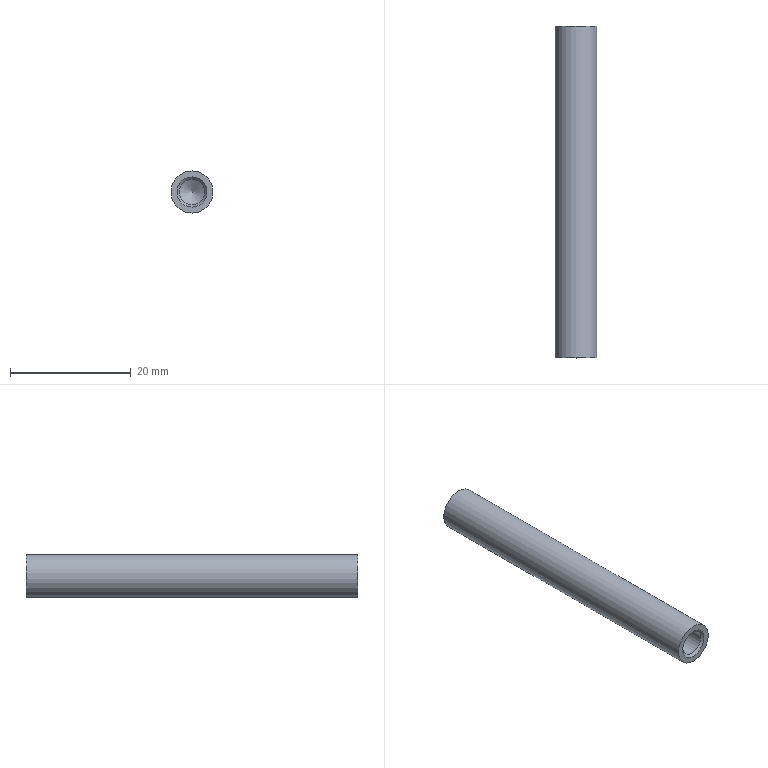Part | STEP file | Coupler copper rod | 1 solid | 9 faces | box 7 x 55 x 7 mm | volume 1826 mm3 | cone 4 | cylinder 3 | plane 2 | commonest cylinder face diameters 4.2 x2 7 x1
STEP:
#1=CARTESIAN_POINT('',(0.,0.,0.));
#2=DIRECTION('',(0.,0.,1.));
#3=DIRECTION('',(1.,0.,0.));
#4=AXIS2_PLACEMENT_3D('',#1,#2,#3);
#5=CARTESIAN_POINT('',(0.,27.5,3.5));
#6=VERTEX_POINT('',#5);
#7=CARTESIAN_POINT('',(0.,27.5,0.));
#8=DIRECTION('',(0.,1.,0.));
#9=DIRECTION('',(0.,0.,1.));
#10=AXIS2_PLACEMENT_3D('',#7,#8,#9);
#11=CIRCLE('',#10,3.5);
#12=CARTESIAN_POINT('',(0.,27.5,0.));
#13=DIRECTION('',(0.,-1.,0.));
#14=DIRECTION('',(0.,0.,-1.));
#15=AXIS2_PLACEMENT_3D('',#12,#13,#14);
#16=CYLINDRICAL_SURFACE('',#15,3.5);
#17=CARTESIAN_POINT('',(9.425,0.));
#18=DIRECTION('',(-1.,0.));
#19=VECTOR('',#18,1.);
#20=LINE('',#17,#19);
#21=(GEOMETRIC_REPRESENTATION_CONTEXT(2)PARAMETRIC_REPRESENTATION_CONTEXT()REPRESENTATION_CONTEXT('',''));
#22=DEFINITIONAL_REPRESENTATION('',(#20),#21);
#23=PCURVE('',#16,#22);
#24=CARTESIAN_POINT('',(0.,27.5,0.));
#25=DIRECTION('',(0.,1.,0.));
#26=DIRECTION('',(0.,0.,1.));
#27=AXIS2_PLACEMENT_3D('',#24,#25,#26);
#28=PLANE('',#27);
#29=CARTESIAN_POINT('',(0.,0.));
#30=DIRECTION('',(1.,0.));
#31=AXIS2_PLACEMENT_2D('',#29,#30);
#32=CIRCLE('',#31,3.5);
#33=(GEOMETRIC_REPRESENTATION_CONTEXT(2)PARAMETRIC_REPRESENTATION_CONTEXT()REPRESENTATION_CONTEXT('',''));
#34=DEFINITIONAL_REPRESENTATION('',(#32),#33);
#35=PCURVE('',#28,#34);
#36=SURFACE_CURVE('',#11,(#23,#35),.PCURVE_S1.);
#37=EDGE_CURVE('',#6,#6,#36,.T.);
#38=ORIENTED_EDGE('',*,*,#37,.F.);
#39=CARTESIAN_POINT('',(0.,-27.5,3.5));
#40=VERTEX_POINT('',#39);
#41=CARTESIAN_POINT('',(0.,27.5,3.5));
#42=CARTESIAN_POINT('',(0.,-27.5,3.5));
#43=B_SPLINE_CURVE_WITH_KNOTS('',1,(#41,#42),.UNSPECIFIED.,.F.,.F.,(2,2),(0.,55.),.PIECEWISE_BEZIER_KNOTS.);
#44=CARTESIAN_POINT('',(9.425,0.));
#45=DIRECTION('',(0.,1.));
#46=VECTOR('',#45,1.);
#47=LINE('',#44,#46);
#48=(GEOMETRIC_REPRESENTATION_CONTEXT(2)PARAMETRIC_REPRESENTATION_CONTEXT()REPRESENTATION_CONTEXT('',''));
#49=DEFINITIONAL_REPRESENTATION('',(#47),#48);
#50=PCURVE('',#16,#49);
#51=CARTESIAN_POINT('',(3.142,0.));
#52=DIRECTION('',(0.,1.));
#53=VECTOR('',#52,1.);
#54=LINE('',#51,#53);
#55=(GEOMETRIC_REPRESENTATION_CONTEXT(2)PARAMETRIC_REPRESENTATION_CONTEXT()REPRESENTATION_CONTEXT('',''));
#56=DEFINITIONAL_REPRESENTATION('',(#54),#55);
#57=PCURVE('',#16,#56);
#58=SEAM_CURVE('',#43,(#50,#57),.PCURVE_S1.);
#59=EDGE_CURVE('',#6,#40,#58,.T.);
#60=ORIENTED_EDGE('',*,*,#59,.T.);
#61=CARTESIAN_POINT('',(0.,-27.5,0.));
#62=DIRECTION('',(0.,1.,0.));
#63=DIRECTION('',(0.,0.,1.));
#64=AXIS2_PLACEMENT_3D('',#61,#62,#63);
#65=CIRCLE('',#64,3.5);
#66=CARTESIAN_POINT('',(9.425,55.));
#67=DIRECTION('',(-1.,0.));
#68=VECTOR('',#67,1.);
#69=LINE('',#66,#68);
#70=(GEOMETRIC_REPRESENTATION_CONTEXT(2)PARAMETRIC_REPRESENTATION_CONTEXT()REPRESENTATION_CONTEXT('',''));
#71=DEFINITIONAL_REPRESENTATION('',(#69),#70);
#72=PCURVE('',#16,#71);
#73=CARTESIAN_POINT('',(0.,-27.5,0.));
#74=DIRECTION('',(0.,1.,0.));
#75=DIRECTION('',(0.,0.,1.));
#76=AXIS2_PLACEMENT_3D('',#73,#74,#75);
#77=PLANE('',#76);
#78=CARTESIAN_POINT('',(0.,0.));
#79=DIRECTION('',(1.,0.));
#80=AXIS2_PLACEMENT_2D('',#78,#79);
#81=CIRCLE('',#80,3.5);
#82=(GEOMETRIC_REPRESENTATION_CONTEXT(2)PARAMETRIC_REPRESENTATION_CONTEXT()REPRESENTATION_CONTEXT('',''));
#83=DEFINITIONAL_REPRESENTATION('',(#81),#82);
#84=PCURVE('',#77,#83);
#85=SURFACE_CURVE('',#65,(#72,#84),.PCURVE_S1.);
#86=EDGE_CURVE('',#40,#40,#85,.T.);
#87=ORIENTED_EDGE('',*,*,#86,.T.);
#88=ORIENTED_EDGE('',*,*,#59,.F.);
#89=EDGE_LOOP('',(#38,#60,#87,#88));
#90=FACE_BOUND('',#89,.T.);
#91=ADVANCED_FACE('',(#90),#16,.T.);
#92=CARTESIAN_POINT('',(0.,27.5,2.5));
#93=VERTEX_POINT('',#92);
#94=CARTESIAN_POINT('',(0.,27.5,0.));
#95=DIRECTION('',(0.,1.,0.));
#96=DIRECTION('',(0.,0.,1.));
#97=AXIS2_PLACEMENT_3D('',#94,#95,#96);
#98=CIRCLE('',#97,2.5);
#99=CARTESIAN_POINT('',(0.,0.));
#100=DIRECTION('',(1.,0.));
#101=AXIS2_PLACEMENT_2D('',#99,#100);
#102=CIRCLE('',#101,2.5);
#103=(GEOMETRIC_REPRESENTATION_CONTEXT(2)PARAMETRIC_REPRESENTATION_CONTEXT()REPRESENTATION_CONTEXT('',''));
#104=DEFINITIONAL_REPRESENTATION('',(#102),#103);
#105=PCURVE('',#28,#104);
#106=CARTESIAN_POINT('',(0.,25.,0.));
#107=DIRECTION('',(0.,1.,0.));
#108=DIRECTION('',(1.,0.,0.));
#109=AXIS2_PLACEMENT_3D('',#106,#107,#108);
#110=CONICAL_SURFACE('',#109,0.,0.7854);
#111=CARTESIAN_POINT('',(4.712,2.5));
#112=DIRECTION('',(1.,0.));
#113=VECTOR('',#112,1.);
#114=LINE('',#111,#113);
#115=(GEOMETRIC_REPRESENTATION_CONTEXT(2)PARAMETRIC_REPRESENTATION_CONTEXT()REPRESENTATION_CONTEXT('',''));
#116=DEFINITIONAL_REPRESENTATION('',(#114),#115);
#117=PCURVE('',#110,#116);
#118=SURFACE_CURVE('',#98,(#105,#117),.PCURVE_S1.);
#119=EDGE_CURVE('',#93,#93,#118,.T.);
#120=ORIENTED_EDGE('',*,*,#119,.F.);
#121=EDGE_LOOP('',(#120));
#122=FACE_BOUND('',#121,.T.);
#123=ORIENTED_EDGE('',*,*,#37,.T.);
#124=EDGE_LOOP('',(#123));
#125=FACE_BOUND('',#124,.T.);
#126=ADVANCED_FACE('',(#122,#125),#28,.T.);
#127=CARTESIAN_POINT('',(0.,-27.5,2.5));
#128=VERTEX_POINT('',#127);
#129=CARTESIAN_POINT('',(0.,-27.5,0.));
#130=DIRECTION('',(0.,1.,0.));
#131=DIRECTION('',(0.,0.,1.));
#132=AXIS2_PLACEMENT_3D('',#129,#130,#131);
#133=CIRCLE('',#132,2.5);
#134=CARTESIAN_POINT('',(0.,0.));
#135=DIRECTION('',(1.,0.));
#136=AXIS2_PLACEMENT_2D('',#134,#135);
#137=CIRCLE('',#136,2.5);
#138=(GEOMETRIC_REPRESENTATION_CONTEXT(2)PARAMETRIC_REPRESENTATION_CONTEXT()REPRESENTATION_CONTEXT('',''));
#139=DEFINITIONAL_REPRESENTATION('',(#137),#138);
#140=PCURVE('',#77,#139);
#141=CARTESIAN_POINT('',(0.,-25.,0.));
#142=DIRECTION('',(0.,-1.,0.));
#143=DIRECTION('',(-1.,0.,0.));
#144=AXIS2_PLACEMENT_3D('',#141,#142,#143);
#145=CONICAL_SURFACE('',#144,0.,0.7854);
#146=CARTESIAN_POINT('',(10.996,2.5));
#147=DIRECTION('',(-1.,0.));
#148=VECTOR('',#147,1.);
#149=LINE('',#146,#148);
#150=(GEOMETRIC_REPRESENTATION_CONTEXT(2)PARAMETRIC_REPRESENTATION_CONTEXT()REPRESENTATION_CONTEXT('',''));
#151=DEFINITIONAL_REPRESENTATION('',(#149),#150);
#152=PCURVE('',#145,#151);
#153=SURFACE_CURVE('',#133,(#140,#152),.PCURVE_S1.);
#154=EDGE_CURVE('',#128,#128,#153,.T.);
#155=ORIENTED_EDGE('',*,*,#154,.T.);
#156=EDGE_LOOP('',(#155));
#157=FACE_BOUND('',#156,.T.);
#158=ORIENTED_EDGE('',*,*,#86,.F.);
#159=EDGE_LOOP('',(#158));
#160=FACE_BOUND('',#159,.T.);
#161=ADVANCED_FACE('',(#157,#160),#77,.F.);
#162=ORIENTED_EDGE('',*,*,#154,.T.);
#163=CARTESIAN_POINT('',(0.,-27.1,2.1));
#164=VERTEX_POINT('',#163);
#165=CARTESIAN_POINT('',(0.,-27.1,2.1));
#166=CARTESIAN_POINT('',(0.,-27.5,2.5));
#167=B_SPLINE_CURVE_WITH_KNOTS('',1,(#165,#166),.UNSPECIFIED.,.F.,.F.,(2,2),(2.97,3.536),.PIECEWISE_BEZIER_KNOTS.);
#168=CARTESIAN_POINT('',(4.712,0.));
#169=DIRECTION('',(0.,1.));
#170=VECTOR('',#169,1.);
#171=LINE('',#168,#170);
#172=(GEOMETRIC_REPRESENTATION_CONTEXT(2)PARAMETRIC_REPRESENTATION_CONTEXT()REPRESENTATION_CONTEXT('',''));
#173=DEFINITIONAL_REPRESENTATION('',(#171),#172);
#174=PCURVE('',#145,#173);
#175=CARTESIAN_POINT('',(10.996,0.));
#176=DIRECTION('',(0.,1.));
#177=VECTOR('',#176,1.);
#178=LINE('',#175,#177);
#179=(GEOMETRIC_REPRESENTATION_CONTEXT(2)PARAMETRIC_REPRESENTATION_CONTEXT()REPRESENTATION_CONTEXT('',''));
#180=DEFINITIONAL_REPRESENTATION('',(#178),#179);
#181=PCURVE('',#145,#180);
#182=SEAM_CURVE('',#167,(#174,#181),.PCURVE_S1.);
#183=EDGE_CURVE('',#164,#128,#182,.T.);
#184=ORIENTED_EDGE('',*,*,#183,.F.);
#185=CARTESIAN_POINT('',(0.,-27.1,-2.1));
#186=VERTEX_POINT('',#185);
#187=CARTESIAN_POINT('',(0.,-27.1,0.));
#188=DIRECTION('',(0.,-1.,0.));
#189=DIRECTION('',(0.,0.,-1.));
#190=AXIS2_PLACEMENT_3D('',#187,#188,#189);
#191=CIRCLE('',#190,2.1);
#192=CARTESIAN_POINT('',(1.571,2.1));
#193=DIRECTION('',(1.,0.));
#194=VECTOR('',#193,1.);
#195=LINE('',#192,#194);
#196=(GEOMETRIC_REPRESENTATION_CONTEXT(2)PARAMETRIC_REPRESENTATION_CONTEXT()REPRESENTATION_CONTEXT('',''));
#197=DEFINITIONAL_REPRESENTATION('',(#195),#196);
#198=PCURVE('',#145,#197);
#199=CARTESIAN_POINT('',(0.,-27.5,0.));
#200=DIRECTION('',(0.,1.,0.));
#201=DIRECTION('',(0.,0.,1.));
#202=AXIS2_PLACEMENT_3D('',#199,#200,#201);
#203=CYLINDRICAL_SURFACE('',#202,2.1);
#204=CARTESIAN_POINT('',(9.425,0.4));
#205=DIRECTION('',(-1.,0.));
#206=VECTOR('',#205,1.);
#207=LINE('',#204,#206);
#208=(GEOMETRIC_REPRESENTATION_CONTEXT(2)PARAMETRIC_REPRESENTATION_CONTEXT()REPRESENTATION_CONTEXT('',''));
#209=DEFINITIONAL_REPRESENTATION('',(#207),#208);
#210=PCURVE('',#203,#209);
#211=SURFACE_CURVE('',#191,(#198,#210),.PCURVE_S1.);
#212=EDGE_CURVE('',#164,#186,#211,.T.);
#213=ORIENTED_EDGE('',*,*,#212,.T.);
#214=CARTESIAN_POINT('',(0.,-27.1,0.));
#215=DIRECTION('',(0.,-1.,0.));
#216=DIRECTION('',(0.,0.,-1.));
#217=AXIS2_PLACEMENT_3D('',#214,#215,#216);
#218=CIRCLE('',#217,2.1);
#219=CARTESIAN_POINT('',(7.854,2.1));
#220=DIRECTION('',(1.,0.));
#221=VECTOR('',#220,1.);
#222=LINE('',#219,#221);
#223=(GEOMETRIC_REPRESENTATION_CONTEXT(2)PARAMETRIC_REPRESENTATION_CONTEXT()REPRESENTATION_CONTEXT('',''));
#224=DEFINITIONAL_REPRESENTATION('',(#222),#223);
#225=PCURVE('',#145,#224);
#226=CARTESIAN_POINT('',(3.142,0.4));
#227=DIRECTION('',(-1.,0.));
#228=VECTOR('',#227,1.);
#229=LINE('',#226,#228);
#230=(GEOMETRIC_REPRESENTATION_CONTEXT(2)PARAMETRIC_REPRESENTATION_CONTEXT()REPRESENTATION_CONTEXT('',''));
#231=DEFINITIONAL_REPRESENTATION('',(#229),#230);
#232=PCURVE('',#203,#231);
#233=SURFACE_CURVE('',#218,(#225,#232),.PCURVE_S1.);
#234=EDGE_CURVE('',#186,#164,#233,.T.);
#235=ORIENTED_EDGE('',*,*,#234,.T.);
#236=ORIENTED_EDGE('',*,*,#183,.T.);
#237=EDGE_LOOP('',(#162,#184,#213,#235,#236));
#238=FACE_BOUND('',#237,.F.);
#239=ADVANCED_FACE('',(#238),#145,.F.);
#240=CARTESIAN_POINT('',(0.,-17.5,-2.1));
#241=VERTEX_POINT('',#240);
#242=CARTESIAN_POINT('',(0.,-17.5,2.1));
#243=VERTEX_POINT('',#242);
#244=CARTESIAN_POINT('',(0.,-17.5,0.));
#245=DIRECTION('',(0.,-1.,0.));
#246=DIRECTION('',(0.,0.,1.));
#247=AXIS2_PLACEMENT_3D('',#244,#245,#246);
#248=CIRCLE('',#247,2.1);
#249=CARTESIAN_POINT('',(0.,-17.5,0.));
#250=DIRECTION('',(0.,-1.,0.));
#251=DIRECTION('',(0.,0.,-1.));
#252=AXIS2_PLACEMENT_3D('',#249,#250,#251);
#253=CONICAL_SURFACE('',#252,2.1,1.03);
#254=CARTESIAN_POINT('',(-3.142,0.));
#255=DIRECTION('',(1.,0.));
#256=VECTOR('',#255,1.);
#257=LINE('',#254,#256);
#258=(GEOMETRIC_REPRESENTATION_CONTEXT(2)PARAMETRIC_REPRESENTATION_CONTEXT()REPRESENTATION_CONTEXT('',''));
#259=DEFINITIONAL_REPRESENTATION('',(#257),#258);
#260=PCURVE('',#253,#259);
#261=CARTESIAN_POINT('',(6.283,10.));
#262=DIRECTION('',(-1.,0.));
#263=VECTOR('',#262,1.);
#264=LINE('',#261,#263);
#265=(GEOMETRIC_REPRESENTATION_CONTEXT(2)PARAMETRIC_REPRESENTATION_CONTEXT()REPRESENTATION_CONTEXT('',''));
#266=DEFINITIONAL_REPRESENTATION('',(#264),#265);
#267=PCURVE('',#203,#266);
#268=SURFACE_CURVE('',#248,(#260,#267),.PCURVE_S1.);
#269=EDGE_CURVE('',#241,#243,#268,.T.);
#270=ORIENTED_EDGE('',*,*,#269,.F.);
#271=CARTESIAN_POINT('',(0.,-16.238,0.));
#272=VERTEX_POINT('',#271);
#273=CARTESIAN_POINT('',(0.,-16.238,0.));
#274=CARTESIAN_POINT('',(0.,-17.5,-2.1));
#275=B_SPLINE_CURVE_WITH_KNOTS('',1,(#273,#274),.UNSPECIFIED.,.F.,.F.,(2,2),(-2.45,0.),.PIECEWISE_BEZIER_KNOTS.);
#276=CARTESIAN_POINT('',(0.,0.));
#277=DIRECTION('',(0.,1.));
#278=VECTOR('',#277,1.);
#279=LINE('',#276,#278);
#280=(GEOMETRIC_REPRESENTATION_CONTEXT(2)PARAMETRIC_REPRESENTATION_CONTEXT()REPRESENTATION_CONTEXT('',''));
#281=DEFINITIONAL_REPRESENTATION('',(#279),#280);
#282=PCURVE('',#253,#281);
#283=CARTESIAN_POINT('',(6.283,0.));
#284=DIRECTION('',(0.,1.));
#285=VECTOR('',#284,1.);
#286=LINE('',#283,#285);
#287=(GEOMETRIC_REPRESENTATION_CONTEXT(2)PARAMETRIC_REPRESENTATION_CONTEXT()REPRESENTATION_CONTEXT('',''));
#288=DEFINITIONAL_REPRESENTATION('',(#286),#287);
#289=PCURVE('',#253,#288);
#290=SEAM_CURVE('',#275,(#282,#289),.PCURVE_S1.);
#291=EDGE_CURVE('',#272,#241,#290,.T.);
#292=ORIENTED_EDGE('',*,*,#291,.F.);
#293=ORIENTED_EDGE('',*,*,#291,.T.);
#294=CARTESIAN_POINT('',(0.,-17.5,0.));
#295=DIRECTION('',(0.,-1.,0.));
#296=DIRECTION('',(0.,0.,1.));
#297=AXIS2_PLACEMENT_3D('',#294,#295,#296);
#298=CIRCLE('',#297,2.1);
#299=CARTESIAN_POINT('',(3.142,0.));
#300=DIRECTION('',(1.,0.));
#301=VECTOR('',#300,1.);
#302=LINE('',#299,#301);
#303=(GEOMETRIC_REPRESENTATION_CONTEXT(2)PARAMETRIC_REPRESENTATION_CONTEXT()REPRESENTATION_CONTEXT('',''));
#304=DEFINITIONAL_REPRESENTATION('',(#302),#303);
#305=PCURVE('',#253,#304);
#306=CARTESIAN_POINT('',(6.283,10.));
#307=DIRECTION('',(-1.,0.));
#308=VECTOR('',#307,1.);
#309=LINE('',#306,#308);
#310=(GEOMETRIC_REPRESENTATION_CONTEXT(2)PARAMETRIC_REPRESENTATION_CONTEXT()REPRESENTATION_CONTEXT('',''));
#311=DEFINITIONAL_REPRESENTATION('',(#309),#310);
#312=PCURVE('',#203,#311);
#313=SURFACE_CURVE('',#298,(#305,#312),.PCURVE_S1.);
#314=EDGE_CURVE('',#243,#241,#313,.T.);
#315=ORIENTED_EDGE('',*,*,#314,.F.);
#316=EDGE_LOOP('',(#270,#292,#293,#315));
#317=FACE_BOUND('',#316,.F.);
#318=ADVANCED_FACE('',(#317),#253,.F.);
#319=ORIENTED_EDGE('',*,*,#212,.F.);
#320=CARTESIAN_POINT('',(0.,-27.1,2.1));
#321=CARTESIAN_POINT('',(0.,-17.5,2.1));
#322=B_SPLINE_CURVE_WITH_KNOTS('',1,(#320,#321),.UNSPECIFIED.,.F.,.F.,(2,2),(0.4,10.),.PIECEWISE_BEZIER_KNOTS.);
#323=CARTESIAN_POINT('',(6.283,0.));
#324=DIRECTION('',(0.,1.));
#325=VECTOR('',#324,1.);
#326=LINE('',#323,#325);
#327=(GEOMETRIC_REPRESENTATION_CONTEXT(2)PARAMETRIC_REPRESENTATION_CONTEXT()REPRESENTATION_CONTEXT('',''));
#328=DEFINITIONAL_REPRESENTATION('',(#326),#327);
#329=PCURVE('',#203,#328);
#330=CARTESIAN_POINT('',(0.,0.));
#331=DIRECTION('',(0.,1.));
#332=VECTOR('',#331,1.);
#333=LINE('',#330,#332);
#334=(GEOMETRIC_REPRESENTATION_CONTEXT(2)PARAMETRIC_REPRESENTATION_CONTEXT()REPRESENTATION_CONTEXT('',''));
#335=DEFINITIONAL_REPRESENTATION('',(#333),#334);
#336=PCURVE('',#203,#335);
#337=SEAM_CURVE('',#322,(#329,#336),.PCURVE_S1.);
#338=EDGE_CURVE('',#164,#243,#337,.T.);
#339=ORIENTED_EDGE('',*,*,#338,.T.);
#340=ORIENTED_EDGE('',*,*,#314,.T.);
#341=ORIENTED_EDGE('',*,*,#269,.T.);
#342=ORIENTED_EDGE('',*,*,#338,.F.);
#343=ORIENTED_EDGE('',*,*,#234,.F.);
#344=EDGE_LOOP('',(#319,#339,#340,#341,#342,#343));
#345=FACE_BOUND('',#344,.F.);
#346=ADVANCED_FACE('',(#345),#203,.F.);
#347=ORIENTED_EDGE('',*,*,#119,.F.);
#348=CARTESIAN_POINT('',(0.,27.1,2.1));
#349=VERTEX_POINT('',#348);
#350=CARTESIAN_POINT('',(0.,27.1,2.1));
#351=CARTESIAN_POINT('',(0.,27.5,2.5));
#352=B_SPLINE_CURVE_WITH_KNOTS('',1,(#350,#351),.UNSPECIFIED.,.F.,.F.,(2,2),(2.97,3.536),.PIECEWISE_BEZIER_KNOTS.);
#353=CARTESIAN_POINT('',(4.712,0.));
#354=DIRECTION('',(0.,1.));
#355=VECTOR('',#354,1.);
#356=LINE('',#353,#355);
#357=(GEOMETRIC_REPRESENTATION_CONTEXT(2)PARAMETRIC_REPRESENTATION_CONTEXT()REPRESENTATION_CONTEXT('',''));
#358=DEFINITIONAL_REPRESENTATION('',(#356),#357);
#359=PCURVE('',#110,#358);
#360=CARTESIAN_POINT('',(10.996,0.));
#361=DIRECTION('',(0.,1.));
#362=VECTOR('',#361,1.);
#363=LINE('',#360,#362);
#364=(GEOMETRIC_REPRESENTATION_CONTEXT(2)PARAMETRIC_REPRESENTATION_CONTEXT()REPRESENTATION_CONTEXT('',''));
#365=DEFINITIONAL_REPRESENTATION('',(#363),#364);
#366=PCURVE('',#110,#365);
#367=SEAM_CURVE('',#352,(#359,#366),.PCURVE_S1.);
#368=EDGE_CURVE('',#349,#93,#367,.T.);
#369=ORIENTED_EDGE('',*,*,#368,.F.);
#370=CARTESIAN_POINT('',(0.,27.1,0.));
#371=DIRECTION('',(0.,1.,0.));
#372=DIRECTION('',(0.,0.,1.));
#373=AXIS2_PLACEMENT_3D('',#370,#371,#372);
#374=CIRCLE('',#373,2.1);
#375=CARTESIAN_POINT('',(4.712,2.1));
#376=DIRECTION('',(1.,0.));
#377=VECTOR('',#376,1.);
#378=LINE('',#375,#377);
#379=(GEOMETRIC_REPRESENTATION_CONTEXT(2)PARAMETRIC_REPRESENTATION_CONTEXT()REPRESENTATION_CONTEXT('',''));
#380=DEFINITIONAL_REPRESENTATION('',(#378),#379);
#381=PCURVE('',#110,#380);
#382=CARTESIAN_POINT('',(0.,27.5,0.));
#383=DIRECTION('',(0.,-1.,0.));
#384=DIRECTION('',(0.,0.,-1.));
#385=AXIS2_PLACEMENT_3D('',#382,#383,#384);
#386=CYLINDRICAL_SURFACE('',#385,2.1);
#387=CARTESIAN_POINT('',(9.425,0.4));
#388=DIRECTION('',(-1.,0.));
#389=VECTOR('',#388,1.);
#390=LINE('',#387,#389);
#391=(GEOMETRIC_REPRESENTATION_CONTEXT(2)PARAMETRIC_REPRESENTATION_CONTEXT()REPRESENTATION_CONTEXT('',''));
#392=DEFINITIONAL_REPRESENTATION('',(#390),#391);
#393=PCURVE('',#386,#392);
#394=SURFACE_CURVE('',#374,(#381,#393),.PCURVE_S1.);
#395=EDGE_CURVE('',#349,#349,#394,.T.);
#396=ORIENTED_EDGE('',*,*,#395,.T.);
#397=ORIENTED_EDGE('',*,*,#368,.T.);
#398=EDGE_LOOP('',(#347,#369,#396,#397));
#399=FACE_BOUND('',#398,.F.);
#400=ADVANCED_FACE('',(#399),#110,.F.);
#401=CARTESIAN_POINT('',(0.,17.5,2.1));
#402=VERTEX_POINT('',#401);
#403=CARTESIAN_POINT('',(0.,17.5,-2.1));
#404=VERTEX_POINT('',#403);
#405=CARTESIAN_POINT('',(0.,17.5,0.));
#406=DIRECTION('',(0.,1.,0.));
#407=DIRECTION('',(0.,0.,-1.));
#408=AXIS2_PLACEMENT_3D('',#405,#406,#407);
#409=CIRCLE('',#408,2.1);
#410=CARTESIAN_POINT('',(0.,17.5,0.));
#411=DIRECTION('',(0.,1.,0.));
#412=DIRECTION('',(0.,0.,1.));
#413=AXIS2_PLACEMENT_3D('',#410,#411,#412);
#414=CONICAL_SURFACE('',#413,2.1,1.03);
#415=CARTESIAN_POINT('',(-3.142,0.));
#416=DIRECTION('',(1.,0.));
#417=VECTOR('',#416,1.);
#418=LINE('',#415,#417);
#419=(GEOMETRIC_REPRESENTATION_CONTEXT(2)PARAMETRIC_REPRESENTATION_CONTEXT()REPRESENTATION_CONTEXT('',''));
#420=DEFINITIONAL_REPRESENTATION('',(#418),#419);
#421=PCURVE('',#414,#420);
#422=CARTESIAN_POINT('',(12.566,10.));
#423=DIRECTION('',(-1.,0.));
#424=VECTOR('',#423,1.);
#425=LINE('',#422,#424);
#426=(GEOMETRIC_REPRESENTATION_CONTEXT(2)PARAMETRIC_REPRESENTATION_CONTEXT()REPRESENTATION_CONTEXT('',''));
#427=DEFINITIONAL_REPRESENTATION('',(#425),#426);
#428=PCURVE('',#386,#427);
#429=SURFACE_CURVE('',#409,(#421,#428),.PCURVE_S1.);
#430=EDGE_CURVE('',#402,#404,#429,.T.);
#431=ORIENTED_EDGE('',*,*,#430,.F.);
#432=CARTESIAN_POINT('',(0.,16.238,0.));
#433=VERTEX_POINT('',#432);
#434=CARTESIAN_POINT('',(0.,16.238,0.));
#435=CARTESIAN_POINT('',(0.,17.5,2.1));
#436=B_SPLINE_CURVE_WITH_KNOTS('',1,(#434,#435),.UNSPECIFIED.,.F.,.F.,(2,2),(-2.45,0.),.PIECEWISE_BEZIER_KNOTS.);
#437=CARTESIAN_POINT('',(0.,0.));
#438=DIRECTION('',(0.,1.));
#439=VECTOR('',#438,1.);
#440=LINE('',#437,#439);
#441=(GEOMETRIC_REPRESENTATION_CONTEXT(2)PARAMETRIC_REPRESENTATION_CONTEXT()REPRESENTATION_CONTEXT('',''));
#442=DEFINITIONAL_REPRESENTATION('',(#440),#441);
#443=PCURVE('',#414,#442);
#444=CARTESIAN_POINT('',(6.283,0.));
#445=DIRECTION('',(0.,1.));
#446=VECTOR('',#445,1.);
#447=LINE('',#444,#446);
#448=(GEOMETRIC_REPRESENTATION_CONTEXT(2)PARAMETRIC_REPRESENTATION_CONTEXT()REPRESENTATION_CONTEXT('',''));
#449=DEFINITIONAL_REPRESENTATION('',(#447),#448);
#450=PCURVE('',#414,#449);
#451=SEAM_CURVE('',#436,(#443,#450),.PCURVE_S1.);
#452=EDGE_CURVE('',#433,#402,#451,.T.);
#453=ORIENTED_EDGE('',*,*,#452,.F.);
#454=ORIENTED_EDGE('',*,*,#452,.T.);
#455=CARTESIAN_POINT('',(0.,17.5,0.));
#456=DIRECTION('',(0.,1.,0.));
#457=DIRECTION('',(0.,0.,-1.));
#458=AXIS2_PLACEMENT_3D('',#455,#456,#457);
#459=CIRCLE('',#458,2.1);
#460=CARTESIAN_POINT('',(3.142,0.));
#461=DIRECTION('',(1.,0.));
#462=VECTOR('',#461,1.);
#463=LINE('',#460,#462);
#464=(GEOMETRIC_REPRESENTATION_CONTEXT(2)PARAMETRIC_REPRESENTATION_CONTEXT()REPRESENTATION_CONTEXT('',''));
#465=DEFINITIONAL_REPRESENTATION('',(#463),#464);
#466=PCURVE('',#414,#465);
#467=CARTESIAN_POINT('',(6.283,10.));
#468=DIRECTION('',(-1.,0.));
#469=VECTOR('',#468,1.);
#470=LINE('',#467,#469);
#471=(GEOMETRIC_REPRESENTATION_CONTEXT(2)PARAMETRIC_REPRESENTATION_CONTEXT()REPRESENTATION_CONTEXT('',''));
#472=DEFINITIONAL_REPRESENTATION('',(#470),#471);
#473=PCURVE('',#386,#472);
#474=SURFACE_CURVE('',#459,(#466,#473),.PCURVE_S1.);
#475=EDGE_CURVE('',#404,#402,#474,.T.);
#476=ORIENTED_EDGE('',*,*,#475,.F.);
#477=EDGE_LOOP('',(#431,#453,#454,#476));
#478=FACE_BOUND('',#477,.F.);
#479=ADVANCED_FACE('',(#478),#414,.F.);
#480=ORIENTED_EDGE('',*,*,#395,.F.);
#481=CARTESIAN_POINT('',(0.,27.1,2.1));
#482=CARTESIAN_POINT('',(0.,17.5,2.1));
#483=B_SPLINE_CURVE_WITH_KNOTS('',1,(#481,#482),.UNSPECIFIED.,.F.,.F.,(2,2),(0.4,10.),.PIECEWISE_BEZIER_KNOTS.);
#484=CARTESIAN_POINT('',(9.425,0.));
#485=DIRECTION('',(0.,1.));
#486=VECTOR('',#485,1.);
#487=LINE('',#484,#486);
#488=(GEOMETRIC_REPRESENTATION_CONTEXT(2)PARAMETRIC_REPRESENTATION_CONTEXT()REPRESENTATION_CONTEXT('',''));
#489=DEFINITIONAL_REPRESENTATION('',(#487),#488);
#490=PCURVE('',#386,#489);
#491=CARTESIAN_POINT('',(3.142,0.));
#492=DIRECTION('',(0.,1.));
#493=VECTOR('',#492,1.);
#494=LINE('',#491,#493);
#495=(GEOMETRIC_REPRESENTATION_CONTEXT(2)PARAMETRIC_REPRESENTATION_CONTEXT()REPRESENTATION_CONTEXT('',''));
#496=DEFINITIONAL_REPRESENTATION('',(#494),#495);
#497=PCURVE('',#386,#496);
#498=SEAM_CURVE('',#483,(#490,#497),.PCURVE_S1.);
#499=EDGE_CURVE('',#349,#402,#498,.T.);
#500=ORIENTED_EDGE('',*,*,#499,.T.);
#501=ORIENTED_EDGE('',*,*,#430,.T.);
#502=ORIENTED_EDGE('',*,*,#475,.T.);
#503=ORIENTED_EDGE('',*,*,#499,.F.);
#504=EDGE_LOOP('',(#480,#500,#501,#502,#503));
#505=FACE_BOUND('',#504,.F.);
#506=ADVANCED_FACE('',(#505),#386,.F.);
#507=CLOSED_SHELL('',(#91,#126,#161,#239,#318,#346,#400,#479,#506));
#508=MANIFOLD_SOLID_BREP('',#507);
#509=(LENGTH_UNIT()NAMED_UNIT(*)SI_UNIT(.MILLI.,.METRE.));
#510=UNCERTAINTY_MEASURE_WITH_UNIT(LENGTH_MEASURE(0.00001),#509,'','');
#511=(NAMED_UNIT(*)PLANE_ANGLE_UNIT()SI_UNIT($,.RADIAN.));
#512=(NAMED_UNIT(*)SI_UNIT($,.STERADIAN.)SOLID_ANGLE_UNIT());
#513=(GEOMETRIC_REPRESENTATION_CONTEXT(3)GLOBAL_UNCERTAINTY_ASSIGNED_CONTEXT((#510))GLOBAL_UNIT_ASSIGNED_CONTEXT((#509,#511,#512))REPRESENTATION_CONTEXT('',''));
#514=ADVANCED_BREP_SHAPE_REPRESENTATION('',(#4,#508),#513);